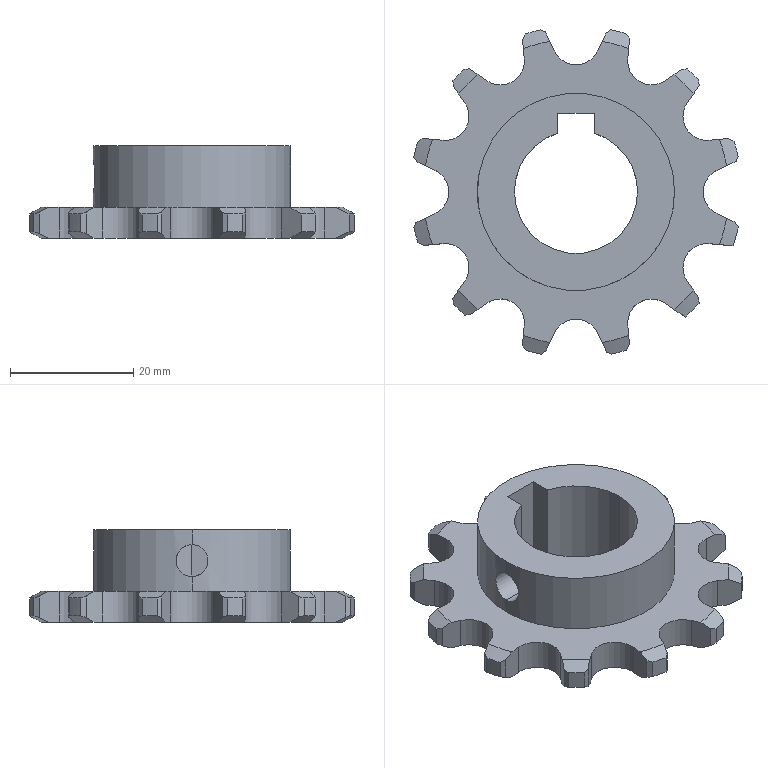Part | NX | features BREP 1 | 1 solid | 112 faces | box 52.696 x 52.696 x 15 mm | volume 11484 mm3 | plane 52 | cylinder 36 | cone 24 | commonest cylinder face diameters 7.77 x17 53.9 x12 20 x3 5.2 x2 32 x2